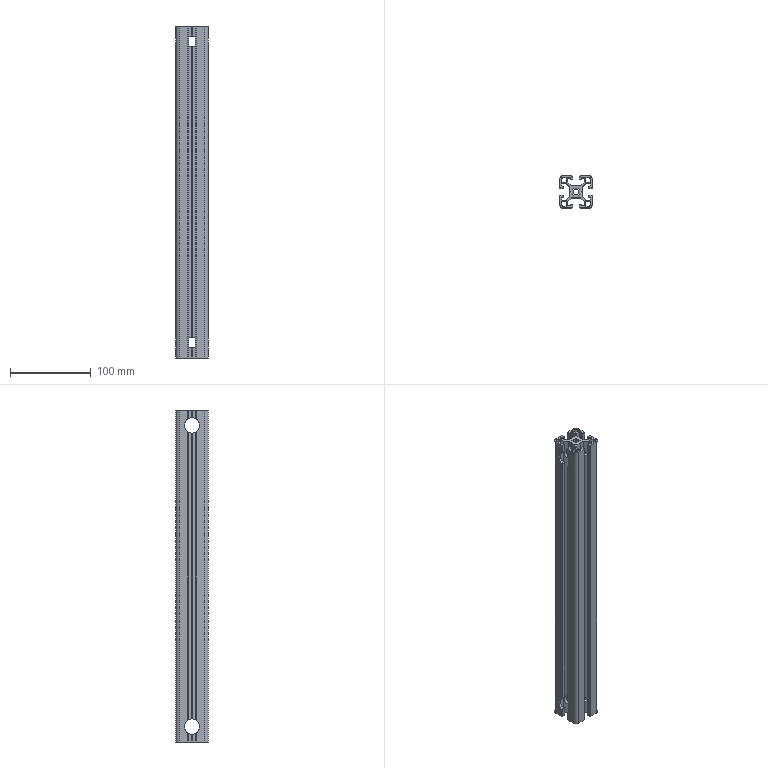Part | SolidWorks | features Extrusion 1, HoleWzd 1 | 1 solid | 273 faces | box 40 x 40 x 410 mm | volume 238068 mm3 | plane 213 | cylinder 60 | commonest cylinder face diameters 2 x16 6.8 x15 19 x12 1 x8 5 x4 9 x4